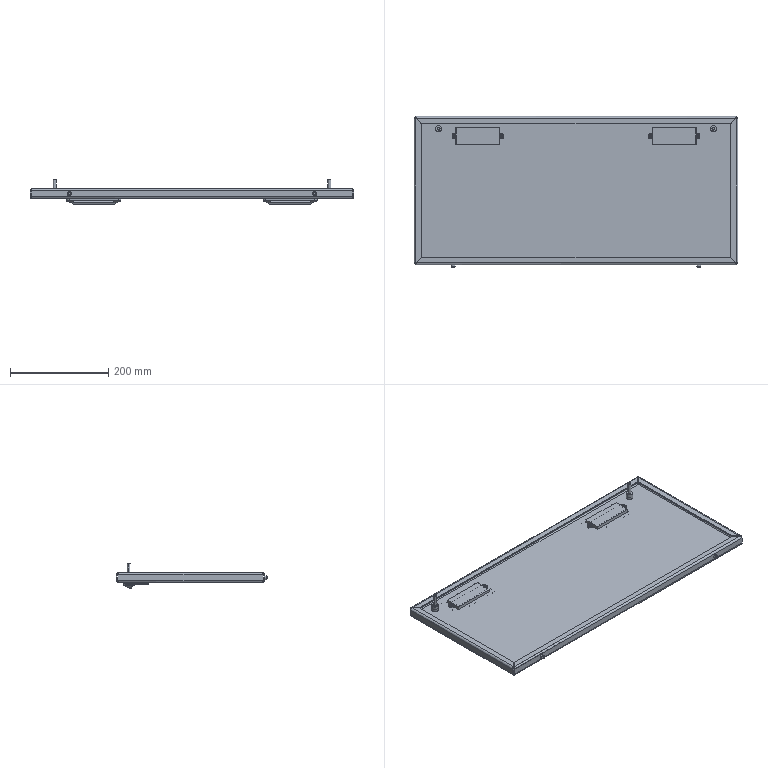Part | NX | features BREP 3 | 5 solids | 422 faces | box 660 x 308 x 51.5 mm | volume 555188 mm3 | plane 216 | cylinder 166 | spline 16 | torus 12 | cone 12 | commonest cylinder face diameters 6 x20 10 x20 4 x16 7 x14 8 x12 8.6 x12